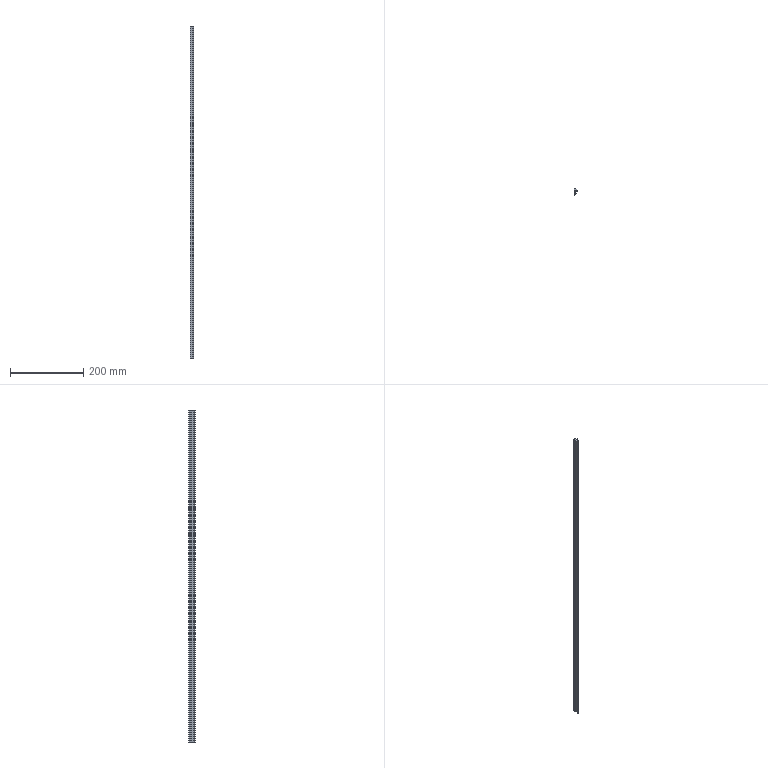Part | SolidWorks | features BaseBody 1, MoveFace 1 | 1 solid | 20 faces | box 10.8 x 17.5 x 907 mm | volume 71472 mm3 | cylinder 11 | plane 9 | commonest cylinder face diameters 1.6 x2 14 x2 0.4 x1 0.6 x1 0.8 x1 2.6 x1
STEP:
#1=CARTESIAN_POINT('',(-3.236,-11.055,807.));
#2=VERTEX_POINT('',#1);
#3=CARTESIAN_POINT('',(-4.3,-10.3,807.));
#4=VERTEX_POINT('',#3);
#5=CARTESIAN_POINT('',(-3.5,-10.3,807.));
#6=DIRECTION('',(0.,0.,-1.));
#7=DIRECTION('',(1.,0.,0.));
#8=AXIS2_PLACEMENT_3D('',#5,#6,#7);
#9=CIRCLE('',#8,0.8);
#10=EDGE_CURVE('',#2,#4,#9,.T.);
#11=ORIENTED_EDGE('',*,*,#10,.T.);
#12=CARTESIAN_POINT('',(-4.3,-10.3,-100.));
#13=VERTEX_POINT('',#12);
#14=CARTESIAN_POINT('',(-4.3,-10.3,-100.));
#15=DIRECTION('',(0.,0.,-1.));
#16=VECTOR('',#15,1000.);
#17=LINE('',#14,#16);
#18=EDGE_CURVE('',#4,#13,#17,.T.);
#19=ORIENTED_EDGE('',*,*,#18,.T.);
#20=CARTESIAN_POINT('',(-3.236,-11.055,-100.));
#21=VERTEX_POINT('',#20);
#22=CARTESIAN_POINT('',(-3.5,-10.3,-100.));
#23=DIRECTION('',(0.,0.,1.));
#24=DIRECTION('',(-1.,0.,0.));
#25=AXIS2_PLACEMENT_3D('',#22,#23,#24);
#26=CIRCLE('',#25,0.8);
#27=EDGE_CURVE('',#13,#21,#26,.T.);
#28=ORIENTED_EDGE('',*,*,#27,.T.);
#29=CARTESIAN_POINT('',(-3.236,-11.055,-100.));
#30=DIRECTION('',(0.,0.,-1.));
#31=VECTOR('',#30,1000.);
#32=LINE('',#29,#31);
#33=EDGE_CURVE('',#2,#21,#32,.T.);
#34=ORIENTED_EDGE('',*,*,#33,.F.);
#35=EDGE_LOOP('',(#11,#19,#28,#34));
#36=FACE_OUTER_BOUND('',#35,.T.);
#37=CARTESIAN_POINT('',(-3.5,-10.3,-100.));
#38=DIRECTION('',(0.,0.,-1.));
#39=DIRECTION('',(-1.,0.,0.));
#40=AXIS2_PLACEMENT_3D('',#37,#38,#39);
#41=CYLINDRICAL_SURFACE('',#40,0.8);
#42=ADVANCED_FACE('',(#36),#41,.T.);
#43=CARTESIAN_POINT('',(1.184,-6.397,-100.));
#44=VERTEX_POINT('',#43);
#45=CARTESIAN_POINT('',(-5.702,-4.29,-100.));
#46=DIRECTION('',(0.,0.,1.));
#47=DIRECTION('',(-1.,0.,0.));
#48=AXIS2_PLACEMENT_3D('',#45,#46,#47);
#49=CIRCLE('',#48,7.201);
#50=EDGE_CURVE('',#21,#44,#49,.T.);
#51=ORIENTED_EDGE('',*,*,#50,.T.);
#52=CARTESIAN_POINT('',(1.184,-6.397,807.));
#53=VERTEX_POINT('',#52);
#54=CARTESIAN_POINT('',(1.184,-6.397,-100.));
#55=DIRECTION('',(0.,0.,1.));
#56=VECTOR('',#55,1000.);
#57=LINE('',#54,#56);
#58=EDGE_CURVE('',#44,#53,#57,.T.);
#59=ORIENTED_EDGE('',*,*,#58,.T.);
#60=CARTESIAN_POINT('',(-5.702,-4.29,807.));
#61=DIRECTION('',(0.,0.,-1.));
#62=DIRECTION('',(1.,0.,0.));
#63=AXIS2_PLACEMENT_3D('',#60,#61,#62);
#64=CIRCLE('',#63,7.201);
#65=EDGE_CURVE('',#53,#2,#64,.T.);
#66=ORIENTED_EDGE('',*,*,#65,.T.);
#67=ORIENTED_EDGE('',*,*,#33,.T.);
#68=EDGE_LOOP('',(#51,#59,#66,#67));
#69=FACE_OUTER_BOUND('',#68,.T.);
#70=CARTESIAN_POINT('',(-5.702,-4.29,-100.));
#71=DIRECTION('',(0.,0.,-1.));
#72=DIRECTION('',(-1.,0.,0.));
#73=AXIS2_PLACEMENT_3D('',#70,#71,#72);
#74=CYLINDRICAL_SURFACE('',#73,7.201);
#75=ADVANCED_FACE('',(#69),#74,.T.);
#76=CARTESIAN_POINT('',(0.9,-6.,-100.));
#77=VERTEX_POINT('',#76);
#78=CARTESIAN_POINT('',(0.9,-6.3,-100.));
#79=DIRECTION('',(0.,0.,1.));
#80=DIRECTION('',(-1.,0.,0.));
#81=AXIS2_PLACEMENT_3D('',#78,#79,#80);
#82=CIRCLE('',#81,0.3);
#83=EDGE_CURVE('',#44,#77,#82,.T.);
#84=ORIENTED_EDGE('',*,*,#83,.T.);
#85=CARTESIAN_POINT('',(0.9,-6.,807.));
#86=VERTEX_POINT('',#85);
#87=CARTESIAN_POINT('',(0.9,-6.,-100.));
#88=DIRECTION('',(0.,0.,1.));
#89=VECTOR('',#88,1000.);
#90=LINE('',#87,#89);
#91=EDGE_CURVE('',#77,#86,#90,.T.);
#92=ORIENTED_EDGE('',*,*,#91,.T.);
#93=CARTESIAN_POINT('',(0.9,-6.3,807.));
#94=DIRECTION('',(0.,0.,-1.));
#95=DIRECTION('',(1.,0.,0.));
#96=AXIS2_PLACEMENT_3D('',#93,#94,#95);
#97=CIRCLE('',#96,0.3);
#98=EDGE_CURVE('',#86,#53,#97,.T.);
#99=ORIENTED_EDGE('',*,*,#98,.T.);
#100=ORIENTED_EDGE('',*,*,#58,.F.);
#101=EDGE_LOOP('',(#84,#92,#99,#100));
#102=FACE_OUTER_BOUND('',#101,.T.);
#103=CARTESIAN_POINT('',(0.9,-6.3,-100.));
#104=DIRECTION('',(0.,0.,-1.));
#105=DIRECTION('',(-1.,0.,0.));
#106=AXIS2_PLACEMENT_3D('',#103,#104,#105);
#107=CYLINDRICAL_SURFACE('',#106,0.3);
#108=ADVANCED_FACE('',(#102),#107,.T.);
#109=CARTESIAN_POINT('',(-2.5,-0.5,-100.));
#110=VERTEX_POINT('',#109);
#111=CARTESIAN_POINT('',(-2.5,-6.153,-100.));
#112=VERTEX_POINT('',#111);
#113=CARTESIAN_POINT('',(-2.5,-6.397,-100.));
#114=DIRECTION('',(0.,-1.,0.));
#115=VECTOR('',#114,1000.);
#116=LINE('',#113,#115);
#117=EDGE_CURVE('',#110,#112,#116,.T.);
#118=ORIENTED_EDGE('',*,*,#117,.F.);
#119=CARTESIAN_POINT('',(-4.2,1.695,-100.));
#120=VERTEX_POINT('',#119);
#121=CARTESIAN_POINT('',(-1.701,1.875,-100.));
#122=DIRECTION('',(0.,0.,1.));
#123=DIRECTION('',(-1.,0.,0.));
#124=AXIS2_PLACEMENT_3D('',#121,#122,#123);
#125=CIRCLE('',#124,2.506);
#126=EDGE_CURVE('',#120,#110,#125,.T.);
#127=ORIENTED_EDGE('',*,*,#126,.F.);
#128=CARTESIAN_POINT('',(-4.2,5.1,-100.));
#129=VERTEX_POINT('',#128);
#130=CARTESIAN_POINT('',(-4.2,-6.397,-100.));
#131=DIRECTION('',(0.,-1.,0.));
#132=VECTOR('',#131,1000.);
#133=LINE('',#130,#132);
#134=EDGE_CURVE('',#129,#120,#133,.T.);
#135=ORIENTED_EDGE('',*,*,#134,.F.);
#136=CARTESIAN_POINT('',(-2.892,6.4,-100.));
#137=VERTEX_POINT('',#136);
#138=CARTESIAN_POINT('',(-2.9,5.1,-100.));
#139=DIRECTION('',(0.,0.,1.));
#140=DIRECTION('',(-1.,0.,0.));
#141=AXIS2_PLACEMENT_3D('',#138,#139,#140);
#142=CIRCLE('',#141,1.3);
#143=EDGE_CURVE('',#137,#129,#142,.T.);
#144=ORIENTED_EDGE('',*,*,#143,.F.);
#145=CARTESIAN_POINT('',(0.5,5.5,-100.));
#146=VERTEX_POINT('',#145);
#147=CARTESIAN_POINT('',(-2.934,-0.5999,-100.));
#148=DIRECTION('',(0.,0.,1.));
#149=DIRECTION('',(-1.,0.,0.));
#150=AXIS2_PLACEMENT_3D('',#147,#148,#149);
#151=CIRCLE('',#150,7.);
#152=EDGE_CURVE('',#146,#137,#151,.T.);
#153=ORIENTED_EDGE('',*,*,#152,.F.);
#154=CARTESIAN_POINT('',(5.5,1.7,-100.));
#155=VERTEX_POINT('',#154);
#156=CARTESIAN_POINT('',(5.5,1.7,-100.));
#157=DIRECTION('',(-0.7962,0.6051,0.));
#158=VECTOR('',#157,1000.);
#159=LINE('',#156,#158);
#160=EDGE_CURVE('',#155,#146,#159,.T.);
#161=ORIENTED_EDGE('',*,*,#160,.F.);
#162=CARTESIAN_POINT('',(6.458,-0.2215,-100.));
#163=VERTEX_POINT('',#162);
#164=CARTESIAN_POINT('',(6.458,-0.2215,-100.));
#165=DIRECTION('',(-0.4462,0.8949,0.));
#166=VECTOR('',#165,1000.);
#167=LINE('',#164,#166);
#168=EDGE_CURVE('',#163,#155,#167,.T.);
#169=ORIENTED_EDGE('',*,*,#168,.F.);
#170=CARTESIAN_POINT('',(5.895,-0.7433,-100.));
#171=VERTEX_POINT('',#170);
#172=CARTESIAN_POINT('',(6.1,-0.4,-100.));
#173=DIRECTION('',(0.,0.,1.));
#174=DIRECTION('',(-1.,0.,0.));
#175=AXIS2_PLACEMENT_3D('',#172,#173,#174);
#176=CIRCLE('',#175,0.4);
#177=EDGE_CURVE('',#171,#163,#176,.T.);
#178=ORIENTED_EDGE('',*,*,#177,.F.);
#179=CARTESIAN_POINT('',(3.,0.,-100.));
#180=VERTEX_POINT('',#179);
#181=CARTESIAN_POINT('',(2.746,-6.995,-100.));
#182=DIRECTION('',(0.,0.,-1.));
#183=DIRECTION('',(-1.,0.,0.));
#184=AXIS2_PLACEMENT_3D('',#181,#182,#183);
#185=CIRCLE('',#184,7.);
#186=EDGE_CURVE('',#180,#171,#185,.T.);
#187=ORIENTED_EDGE('',*,*,#186,.F.);
#188=CARTESIAN_POINT('',(0.,0.,-100.));
#189=VERTEX_POINT('',#188);
#190=CARTESIAN_POINT('',(-6.814,0.,-100.));
#191=DIRECTION('',(1.,0.,0.));
#192=VECTOR('',#191,1000.);
#193=LINE('',#190,#192);
#194=EDGE_CURVE('',#189,#180,#193,.T.);
#195=ORIENTED_EDGE('',*,*,#194,.F.);
#196=CARTESIAN_POINT('',(0.,-5.8,-100.));
#197=VERTEX_POINT('',#196);
#198=CARTESIAN_POINT('',(0.,-6.397,-100.));
#199=DIRECTION('',(0.,1.,0.));
#200=VECTOR('',#199,1000.);
#201=LINE('',#198,#200);
#202=EDGE_CURVE('',#197,#189,#201,.T.);
#203=ORIENTED_EDGE('',*,*,#202,.F.);
#204=CARTESIAN_POINT('',(0.2,-6.,-100.));
#205=VERTEX_POINT('',#204);
#206=CARTESIAN_POINT('',(0.2,-5.8,-100.));
#207=DIRECTION('',(0.,0.,1.));
#208=DIRECTION('',(-1.,0.,0.));
#209=AXIS2_PLACEMENT_3D('',#206,#207,#208);
#210=CIRCLE('',#209,0.2);
#211=EDGE_CURVE('',#197,#205,#210,.T.);
#212=ORIENTED_EDGE('',*,*,#211,.T.);
#213=CARTESIAN_POINT('',(-6.814,-6.,-100.));
#214=DIRECTION('',(-1.,0.,0.));
#215=VECTOR('',#214,1000.);
#216=LINE('',#213,#215);
#217=EDGE_CURVE('',#77,#205,#216,.T.);
#218=ORIENTED_EDGE('',*,*,#217,.F.);
#219=ORIENTED_EDGE('',*,*,#83,.F.);
#220=ORIENTED_EDGE('',*,*,#50,.F.);
#221=ORIENTED_EDGE('',*,*,#27,.F.);
#222=CARTESIAN_POINT('',(-3.998,-9.674,-100.));
#223=VERTEX_POINT('',#222);
#224=CARTESIAN_POINT('',(-3.5,-10.3,-100.));
#225=DIRECTION('',(0.,0.,1.));
#226=DIRECTION('',(-1.,0.,0.));
#227=AXIS2_PLACEMENT_3D('',#224,#225,#226);
#228=CIRCLE('',#227,0.8);
#229=EDGE_CURVE('',#223,#13,#228,.T.);
#230=ORIENTED_EDGE('',*,*,#229,.F.);
#231=CARTESIAN_POINT('',(-6.814,-6.397,-100.));
#232=DIRECTION('',(0.,0.,-1.));
#233=DIRECTION('',(-1.,0.,0.));
#234=AXIS2_PLACEMENT_3D('',#231,#232,#233);
#235=CIRCLE('',#234,4.321);
#236=EDGE_CURVE('',#112,#223,#235,.T.);
#237=ORIENTED_EDGE('',*,*,#236,.F.);
#238=EDGE_LOOP('',(#118,#127,#135,#144,#153,#161,#169,#178,#187,#195,#203,#212,#218,#219,#220,#221,#230,#237));
#239=FACE_OUTER_BOUND('',#238,.T.);
#240=CARTESIAN_POINT('',(-6.814,-6.397,-100.));
#241=DIRECTION('',(0.,0.,1.));
#242=DIRECTION('',(1.,0.,0.));
#243=AXIS2_PLACEMENT_3D('',#240,#241,#242);
#244=PLANE('',#243);
#245=ADVANCED_FACE('',(#239),#244,.F.);
#246=ORIENTED_EDGE('',*,*,#18,.F.);
#247=CARTESIAN_POINT('',(-3.998,-9.674,807.));
#248=VERTEX_POINT('',#247);
#249=CARTESIAN_POINT('',(-3.5,-10.3,807.));
#250=DIRECTION('',(0.,0.,-1.));
#251=DIRECTION('',(1.,0.,0.));
#252=AXIS2_PLACEMENT_3D('',#249,#250,#251);
#253=CIRCLE('',#252,0.8);
#254=EDGE_CURVE('',#4,#248,#253,.T.);
#255=ORIENTED_EDGE('',*,*,#254,.T.);
#256=CARTESIAN_POINT('',(-3.998,-9.674,-100.));
#257=DIRECTION('',(0.,0.,-1.));
#258=VECTOR('',#257,1000.);
#259=LINE('',#256,#258);
#260=EDGE_CURVE('',#248,#223,#259,.T.);
#261=ORIENTED_EDGE('',*,*,#260,.T.);
#262=ORIENTED_EDGE('',*,*,#229,.T.);
#263=EDGE_LOOP('',(#246,#255,#261,#262));
#264=FACE_OUTER_BOUND('',#263,.T.);
#265=CARTESIAN_POINT('',(-3.5,-10.3,-100.));
#266=DIRECTION('',(0.,0.,-1.));
#267=DIRECTION('',(-1.,0.,0.));
#268=AXIS2_PLACEMENT_3D('',#265,#266,#267);
#269=CYLINDRICAL_SURFACE('',#268,0.8);
#270=ADVANCED_FACE('',(#264),#269,.T.);
#271=CARTESIAN_POINT('',(-4.2,1.695,807.));
#272=VERTEX_POINT('',#271);
#273=CARTESIAN_POINT('',(-2.5,-0.5,807.));
#274=VERTEX_POINT('',#273);
#275=CARTESIAN_POINT('',(-1.701,1.875,807.));
#276=DIRECTION('',(0.,0.,1.));
#277=DIRECTION('',(1.,0.,0.));
#278=AXIS2_PLACEMENT_3D('',#275,#276,#277);
#279=CIRCLE('',#278,2.506);
#280=EDGE_CURVE('',#272,#274,#279,.T.);
#281=ORIENTED_EDGE('',*,*,#280,.T.);
#282=CARTESIAN_POINT('',(-2.5,-6.153,807.));
#283=VERTEX_POINT('',#282);
#284=CARTESIAN_POINT('',(-2.5,-6.397,807.));
#285=DIRECTION('',(0.,-1.,0.));
#286=VECTOR('',#285,1000.);
#287=LINE('',#284,#286);
#288=EDGE_CURVE('',#274,#283,#287,.T.);
#289=ORIENTED_EDGE('',*,*,#288,.T.);
#290=CARTESIAN_POINT('',(-6.814,-6.397,807.));
#291=DIRECTION('',(0.,0.,-1.));
#292=DIRECTION('',(1.,0.,0.));
#293=AXIS2_PLACEMENT_3D('',#290,#291,#292);
#294=CIRCLE('',#293,4.321);
#295=EDGE_CURVE('',#283,#248,#294,.T.);
#296=ORIENTED_EDGE('',*,*,#295,.T.);
#297=ORIENTED_EDGE('',*,*,#254,.F.);
#298=ORIENTED_EDGE('',*,*,#10,.F.);
#299=ORIENTED_EDGE('',*,*,#65,.F.);
#300=ORIENTED_EDGE('',*,*,#98,.F.);
#301=CARTESIAN_POINT('',(0.2,-6.,807.));
#302=VERTEX_POINT('',#301);
#303=CARTESIAN_POINT('',(-6.814,-6.,807.));
#304=DIRECTION('',(-1.,0.,0.));
#305=VECTOR('',#304,1000.);
#306=LINE('',#303,#305);
#307=EDGE_CURVE('',#86,#302,#306,.T.);
#308=ORIENTED_EDGE('',*,*,#307,.T.);
#309=CARTESIAN_POINT('',(0.,-5.8,807.));
#310=VERTEX_POINT('',#309);
#311=CARTESIAN_POINT('',(0.2,-5.8,807.));
#312=DIRECTION('',(0.,0.,-1.));
#313=DIRECTION('',(1.,0.,0.));
#314=AXIS2_PLACEMENT_3D('',#311,#312,#313);
#315=CIRCLE('',#314,0.2);
#316=EDGE_CURVE('',#302,#310,#315,.T.);
#317=ORIENTED_EDGE('',*,*,#316,.T.);
#318=CARTESIAN_POINT('',(0.,0.,807.));
#319=VERTEX_POINT('',#318);
#320=CARTESIAN_POINT('',(0.,-6.397,807.));
#321=DIRECTION('',(0.,1.,0.));
#322=VECTOR('',#321,1000.);
#323=LINE('',#320,#322);
#324=EDGE_CURVE('',#310,#319,#323,.T.);
#325=ORIENTED_EDGE('',*,*,#324,.T.);
#326=CARTESIAN_POINT('',(3.,0.,807.));
#327=VERTEX_POINT('',#326);
#328=CARTESIAN_POINT('',(-6.814,0.,807.));
#329=DIRECTION('',(1.,0.,0.));
#330=VECTOR('',#329,1000.);
#331=LINE('',#328,#330);
#332=EDGE_CURVE('',#319,#327,#331,.T.);
#333=ORIENTED_EDGE('',*,*,#332,.T.);
#334=CARTESIAN_POINT('',(5.895,-0.7433,807.));
#335=VERTEX_POINT('',#334);
#336=CARTESIAN_POINT('',(2.746,-6.995,807.));
#337=DIRECTION('',(0.,0.,-1.));
#338=DIRECTION('',(1.,0.,0.));
#339=AXIS2_PLACEMENT_3D('',#336,#337,#338);
#340=CIRCLE('',#339,7.);
#341=EDGE_CURVE('',#327,#335,#340,.T.);
#342=ORIENTED_EDGE('',*,*,#341,.T.);
#343=CARTESIAN_POINT('',(6.458,-0.2215,807.));
#344=VERTEX_POINT('',#343);
#345=CARTESIAN_POINT('',(6.1,-0.4,807.));
#346=DIRECTION('',(0.,0.,-1.));
#347=DIRECTION('',(1.,0.,0.));
#348=AXIS2_PLACEMENT_3D('',#345,#346,#347);
#349=CIRCLE('',#348,0.4);
#350=EDGE_CURVE('',#344,#335,#349,.T.);
#351=ORIENTED_EDGE('',*,*,#350,.F.);
#352=CARTESIAN_POINT('',(5.5,1.7,807.));
#353=VERTEX_POINT('',#352);
#354=CARTESIAN_POINT('',(6.282,0.1323,807.));
#355=DIRECTION('',(-0.4462,0.8949,0.));
#356=VECTOR('',#355,1000.);
#357=LINE('',#354,#356);
#358=EDGE_CURVE('',#344,#353,#357,.T.);
#359=ORIENTED_EDGE('',*,*,#358,.T.);
#360=CARTESIAN_POINT('',(0.5,5.5,807.));
#361=VERTEX_POINT('',#360);
#362=CARTESIAN_POINT('',(1.595,4.668,807.));
#363=DIRECTION('',(-0.7962,0.6051,0.));
#364=VECTOR('',#363,1000.);
#365=LINE('',#362,#364);
#366=EDGE_CURVE('',#353,#361,#365,.T.);
#367=ORIENTED_EDGE('',*,*,#366,.T.);
#368=CARTESIAN_POINT('',(-2.892,6.4,807.));
#369=VERTEX_POINT('',#368);
#370=CARTESIAN_POINT('',(-2.934,-0.5999,807.));
#371=DIRECTION('',(0.,0.,1.));
#372=DIRECTION('',(1.,0.,0.));
#373=AXIS2_PLACEMENT_3D('',#370,#371,#372);
#374=CIRCLE('',#373,7.);
#375=EDGE_CURVE('',#361,#369,#374,.T.);
#376=ORIENTED_EDGE('',*,*,#375,.T.);
#377=CARTESIAN_POINT('',(-4.2,5.1,807.));
#378=VERTEX_POINT('',#377);
#379=CARTESIAN_POINT('',(-2.9,5.1,807.));
#380=DIRECTION('',(0.,0.,1.));
#381=DIRECTION('',(1.,0.,0.));
#382=AXIS2_PLACEMENT_3D('',#379,#380,#381);
#383=CIRCLE('',#382,1.3);
#384=EDGE_CURVE('',#369,#378,#383,.T.);
#385=ORIENTED_EDGE('',*,*,#384,.T.);
#386=CARTESIAN_POINT('',(-4.2,-6.397,807.));
#387=DIRECTION('',(0.,-1.,0.));
#388=VECTOR('',#387,1000.);
#389=LINE('',#386,#388);
#390=EDGE_CURVE('',#378,#272,#389,.T.);
#391=ORIENTED_EDGE('',*,*,#390,.T.);
#392=EDGE_LOOP('',(#281,#289,#296,#297,#298,#299,#300,#308,#317,#325,#333,#342,#351,#359,#367,#376,#385,#391));
#393=FACE_OUTER_BOUND('',#392,.T.);
#394=CARTESIAN_POINT('',(-6.814,-6.397,807.));
#395=DIRECTION('',(0.,0.,1.));
#396=DIRECTION('',(1.,0.,0.));
#397=AXIS2_PLACEMENT_3D('',#394,#395,#396);
#398=PLANE('',#397);
#399=ADVANCED_FACE('',(#393),#398,.T.);
#400=ORIENTED_EDGE('',*,*,#217,.T.);
#401=CARTESIAN_POINT('',(0.2,-6.,-100.));
#402=DIRECTION('',(0.,0.,1.));
#403=VECTOR('',#402,1000.);
#404=LINE('',#401,#403);
#405=EDGE_CURVE('',#205,#302,#404,.T.);
#406=ORIENTED_EDGE('',*,*,#405,.T.);
#407=ORIENTED_EDGE('',*,*,#307,.F.);
#408=ORIENTED_EDGE('',*,*,#91,.F.);
#409=EDGE_LOOP('',(#400,#406,#407,#408));
#410=FACE_OUTER_BOUND('',#409,.T.);
#411=CARTESIAN_POINT('',(0.9,-6.,-100.));
#412=DIRECTION('',(0.,1.,0.));
#413=DIRECTION('',(0.,0.,1.));
#414=AXIS2_PLACEMENT_3D('',#411,#412,#413);
#415=PLANE('',#414);
#416=ADVANCED_FACE('',(#410),#415,.T.);
#417=CARTESIAN_POINT('',(-2.5,-6.153,-100.));
#418=DIRECTION('',(0.,0.,1.));
#419=VECTOR('',#418,1000.);
#420=LINE('',#417,#419);
#421=EDGE_CURVE('',#112,#283,#420,.T.);
#422=ORIENTED_EDGE('',*,*,#421,.F.);
#423=ORIENTED_EDGE('',*,*,#236,.T.);
#424=ORIENTED_EDGE('',*,*,#260,.F.);
#425=ORIENTED_EDGE('',*,*,#295,.F.);
#426=EDGE_LOOP('',(#422,#423,#424,#425));
#427=FACE_OUTER_BOUND('',#426,.T.);
#428=CARTESIAN_POINT('',(-6.814,-6.397,-100.));
#429=DIRECTION('',(0.,0.,-1.));
#430=DIRECTION('',(-1.,0.,0.));
#431=AXIS2_PLACEMENT_3D('',#428,#429,#430);
#432=CYLINDRICAL_SURFACE('',#431,4.321);
#433=ADVANCED_FACE('',(#427),#432,.F.);
#434=ORIENTED_EDGE('',*,*,#117,.T.);
#435=ORIENTED_EDGE('',*,*,#421,.T.);
#436=ORIENTED_EDGE('',*,*,#288,.F.);
#437=CARTESIAN_POINT('',(-2.5,-0.5,-100.));
#438=DIRECTION('',(0.,0.,-1.));
#439=VECTOR('',#438,1000.);
#440=LINE('',#437,#439);
#441=EDGE_CURVE('',#274,#110,#440,.T.);
#442=ORIENTED_EDGE('',*,*,#441,.T.);
#443=EDGE_LOOP('',(#434,#435,#436,#442));
#444=FACE_OUTER_BOUND('',#443,.T.);
#445=CARTESIAN_POINT('',(-2.5,-0.5,-100.));
#446=DIRECTION('',(-1.,0.,0.));
#447=DIRECTION('',(0.,0.,1.));
#448=AXIS2_PLACEMENT_3D('',#445,#446,#447);
#449=PLANE('',#448);
#450=ADVANCED_FACE('',(#444),#449,.T.);
#451=ORIENTED_EDGE('',*,*,#126,.T.);
#452=ORIENTED_EDGE('',*,*,#441,.F.);
#453=ORIENTED_EDGE('',*,*,#280,.F.);
#454=CARTESIAN_POINT('',(-4.2,1.695,-100.));
#455=DIRECTION('',(0.,0.,-1.));
#456=VECTOR('',#455,1000.);
#457=LINE('',#454,#456);
#458=EDGE_CURVE('',#272,#120,#457,.T.);
#459=ORIENTED_EDGE('',*,*,#458,.T.);
#460=EDGE_LOOP('',(#451,#452,#453,#459));
#461=FACE_OUTER_BOUND('',#460,.T.);
#462=CARTESIAN_POINT('',(-1.701,1.875,-100.));
#463=DIRECTION('',(0.,0.,-1.));
#464=DIRECTION('',(-1.,0.,0.));
#465=AXIS2_PLACEMENT_3D('',#462,#463,#464);
#466=CYLINDRICAL_SURFACE('',#465,2.506);
#467=ADVANCED_FACE('',(#461),#466,.T.);
#468=ORIENTED_EDGE('',*,*,#134,.T.);
#469=ORIENTED_EDGE('',*,*,#458,.F.);
#470=ORIENTED_EDGE('',*,*,#390,.F.);
#471=CARTESIAN_POINT('',(-4.2,5.1,-100.));
#472=DIRECTION('',(0.,0.,-1.));
#473=VECTOR('',#472,1000.);
#474=LINE('',#471,#473);
#475=EDGE_CURVE('',#378,#129,#474,.T.);
#476=ORIENTED_EDGE('',*,*,#475,.T.);
#477=EDGE_LOOP('',(#468,#469,#470,#476));
#478=FACE_OUTER_BOUND('',#477,.T.);
#479=CARTESIAN_POINT('',(-4.2,5.1,-100.));
#480=DIRECTION('',(-1.,0.,0.));
#481=DIRECTION('',(0.,0.,1.));
#482=AXIS2_PLACEMENT_3D('',#479,#480,#481);
#483=PLANE('',#482);
#484=ADVANCED_FACE('',(#478),#483,.T.);
#485=ORIENTED_EDGE('',*,*,#143,.T.);
#486=ORIENTED_EDGE('',*,*,#475,.F.);
#487=ORIENTED_EDGE('',*,*,#384,.F.);
#488=CARTESIAN_POINT('',(-2.892,6.4,-100.));
#489=DIRECTION('',(0.,0.,-1.));
#490=VECTOR('',#489,1000.);
#491=LINE('',#488,#490);
#492=EDGE_CURVE('',#369,#137,#491,.T.);
#493=ORIENTED_EDGE('',*,*,#492,.T.);
#494=EDGE_LOOP('',(#485,#486,#487,#493));
#495=FACE_OUTER_BOUND('',#494,.T.);
#496=CARTESIAN_POINT('',(-2.9,5.1,-100.));
#497=DIRECTION('',(0.,0.,-1.));
#498=DIRECTION('',(-1.,0.,0.));
#499=AXIS2_PLACEMENT_3D('',#496,#497,#498);
#500=CYLINDRICAL_SURFACE('',#499,1.3);
#501=ADVANCED_FACE('',(#495),#500,.T.);
#502=ORIENTED_EDGE('',*,*,#152,.T.);
#503=ORIENTED_EDGE('',*,*,#492,.F.);
#504=ORIENTED_EDGE('',*,*,#375,.F.);
#505=CARTESIAN_POINT('',(0.5,5.5,-100.));
#506=DIRECTION('',(0.,0.,-1.));
#507=VECTOR('',#506,1000.);
#508=LINE('',#505,#507);
#509=EDGE_CURVE('',#361,#146,#508,.T.);
#510=ORIENTED_EDGE('',*,*,#509,.T.);
#511=EDGE_LOOP('',(#502,#503,#504,#510));
#512=FACE_OUTER_BOUND('',#511,.T.);
#513=CARTESIAN_POINT('',(-2.934,-0.5999,-100.));
#514=DIRECTION('',(0.,0.,-1.));
#515=DIRECTION('',(-1.,0.,0.));
#516=AXIS2_PLACEMENT_3D('',#513,#514,#515);
#517=CYLINDRICAL_SURFACE('',#516,7.);
#518=ADVANCED_FACE('',(#512),#517,.T.);
#519=ORIENTED_EDGE('',*,*,#160,.T.);
#520=ORIENTED_EDGE('',*,*,#509,.F.);
#521=ORIENTED_EDGE('',*,*,#366,.F.);
#522=CARTESIAN_POINT('',(5.5,1.7,-100.));
#523=DIRECTION('',(0.,0.,-1.));
#524=VECTOR('',#523,1000.);
#525=LINE('',#522,#524);
#526=EDGE_CURVE('',#353,#155,#525,.T.);
#527=ORIENTED_EDGE('',*,*,#526,.T.);
#528=EDGE_LOOP('',(#519,#520,#521,#527));
#529=FACE_OUTER_BOUND('',#528,.T.);
#530=CARTESIAN_POINT('',(5.5,1.7,-100.));
#531=DIRECTION('',(0.6051,0.7962,0.));
#532=DIRECTION('',(-0.7962,0.6051,0.));
#533=AXIS2_PLACEMENT_3D('',#530,#531,#532);
#534=PLANE('',#533);
#535=ADVANCED_FACE('',(#529),#534,.T.);
#536=ORIENTED_EDGE('',*,*,#168,.T.);
#537=ORIENTED_EDGE('',*,*,#526,.F.);
#538=ORIENTED_EDGE('',*,*,#358,.F.);
#539=CARTESIAN_POINT('',(6.458,-0.2215,-100.));
#540=DIRECTION('',(0.,0.,-1.));
#541=VECTOR('',#540,1000.);
#542=LINE('',#539,#541);
#543=EDGE_CURVE('',#344,#163,#542,.T.);
#544=ORIENTED_EDGE('',*,*,#543,.T.);
#545=EDGE_LOOP('',(#536,#537,#538,#544));
#546=FACE_OUTER_BOUND('',#545,.T.);
#547=CARTESIAN_POINT('',(6.458,-0.2215,-100.));
#548=DIRECTION('',(0.8949,0.4462,0.));
#549=DIRECTION('',(-0.4462,0.8949,0.));
#550=AXIS2_PLACEMENT_3D('',#547,#548,#549);
#551=PLANE('',#550);
#552=ADVANCED_FACE('',(#546),#551,.T.);
#553=CARTESIAN_POINT('',(3.,0.,-100.));
#554=DIRECTION('',(0.,0.,1.));
#555=VECTOR('',#554,1000.);
#556=LINE('',#553,#555);
#557=EDGE_CURVE('',#180,#327,#556,.T.);
#558=ORIENTED_EDGE('',*,*,#557,.F.);
#559=ORIENTED_EDGE('',*,*,#186,.T.);
#560=CARTESIAN_POINT('',(5.895,-0.7433,-100.));
#561=DIRECTION('',(0.,0.,-1.));
#562=VECTOR('',#561,1000.);
#563=LINE('',#560,#562);
#564=EDGE_CURVE('',#335,#171,#563,.T.);
#565=ORIENTED_EDGE('',*,*,#564,.F.);
#566=ORIENTED_EDGE('',*,*,#341,.F.);
#567=EDGE_LOOP('',(#558,#559,#565,#566));
#568=FACE_OUTER_BOUND('',#567,.T.);
#569=CARTESIAN_POINT('',(2.746,-6.995,-100.));
#570=DIRECTION('',(0.,0.,-1.));
#571=DIRECTION('',(-1.,0.,0.));
#572=AXIS2_PLACEMENT_3D('',#569,#570,#571);
#573=CYLINDRICAL_SURFACE('',#572,7.);
#574=ADVANCED_FACE('',(#568),#573,.F.);
#575=ORIENTED_EDGE('',*,*,#194,.T.);
#576=ORIENTED_EDGE('',*,*,#557,.T.);
#577=ORIENTED_EDGE('',*,*,#332,.F.);
#578=CARTESIAN_POINT('',(0.,0.,-100.));
#579=DIRECTION('',(0.,0.,-1.));
#580=VECTOR('',#579,1000.);
#581=LINE('',#578,#580);
#582=EDGE_CURVE('',#319,#189,#581,.T.);
#583=ORIENTED_EDGE('',*,*,#582,.T.);
#584=EDGE_LOOP('',(#575,#576,#577,#583));
#585=FACE_OUTER_BOUND('',#584,.T.);
#586=CARTESIAN_POINT('',(0.,0.,-100.));
#587=DIRECTION('',(0.,-1.,0.));
#588=DIRECTION('',(0.,0.,-1.));
#589=AXIS2_PLACEMENT_3D('',#586,#587,#588);
#590=PLANE('',#589);
#591=ADVANCED_FACE('',(#585),#590,.T.);
#592=ORIENTED_EDGE('',*,*,#202,.T.);
#593=ORIENTED_EDGE('',*,*,#582,.F.);
#594=ORIENTED_EDGE('',*,*,#324,.F.);
#595=CARTESIAN_POINT('',(0.,-5.8,-100.));
#596=DIRECTION('',(0.,0.,-1.));
#597=VECTOR('',#596,1000.);
#598=LINE('',#595,#597);
#599=EDGE_CURVE('',#310,#197,#598,.T.);
#600=ORIENTED_EDGE('',*,*,#599,.T.);
#601=EDGE_LOOP('',(#592,#593,#594,#600));
#602=FACE_OUTER_BOUND('',#601,.T.);
#603=CARTESIAN_POINT('',(0.,-5.8,-100.));
#604=DIRECTION('',(1.,0.,0.));
#605=DIRECTION('',(0.,0.,-1.));
#606=AXIS2_PLACEMENT_3D('',#603,#604,#605);
#607=PLANE('',#606);
#608=ADVANCED_FACE('',(#602),#607,.T.);
#609=ORIENTED_EDGE('',*,*,#405,.F.);
#610=ORIENTED_EDGE('',*,*,#211,.F.);
#611=ORIENTED_EDGE('',*,*,#599,.F.);
#612=ORIENTED_EDGE('',*,*,#316,.F.);
#613=EDGE_LOOP('',(#609,#610,#611,#612));
#614=FACE_OUTER_BOUND('',#613,.T.);
#615=CARTESIAN_POINT('',(0.2,-5.8,-100.));
#616=DIRECTION('',(0.,0.,-1.));
#617=DIRECTION('',(-1.,0.,0.));
#618=AXIS2_PLACEMENT_3D('',#615,#616,#617);
#619=CYLINDRICAL_SURFACE('',#618,0.2);
#620=ADVANCED_FACE('',(#614),#619,.F.);
#621=ORIENTED_EDGE('',*,*,#177,.T.);
#622=ORIENTED_EDGE('',*,*,#543,.F.);
#623=ORIENTED_EDGE('',*,*,#350,.T.);
#624=ORIENTED_EDGE('',*,*,#564,.T.);
#625=EDGE_LOOP('',(#621,#622,#623,#624));
#626=FACE_OUTER_BOUND('',#625,.T.);
#627=CARTESIAN_POINT('',(6.1,-0.4,-100.));
#628=DIRECTION('',(0.,0.,-1.));
#629=DIRECTION('',(-1.,0.,0.));
#630=AXIS2_PLACEMENT_3D('',#627,#628,#629);
#631=CYLINDRICAL_SURFACE('',#630,0.4);
#632=ADVANCED_FACE('',(#626),#631,.T.);
#633=CLOSED_SHELL('',(#42,#75,#108,#245,#270,#399,#416,#433,#450,#467,#484,#501,#518,#535,#552,#574,#591,#608,#620,#632));
#634=MANIFOLD_SOLID_BREP('',#633);
#635=CARTESIAN_POINT('',(0.,0.,0.));
#636=DIRECTION('',(0.,0.,1.));
#637=DIRECTION('',(1.,0.,0.));
#638=AXIS2_PLACEMENT_3D('',#635,#636,#637);
#639=(LENGTH_UNIT()NAMED_UNIT(*)SI_UNIT(.MILLI.,.METRE.));
#640=UNCERTAINTY_MEASURE_WITH_UNIT(LENGTH_MEASURE(0.00001),#639,'','');
#641=(NAMED_UNIT(*)PLANE_ANGLE_UNIT()SI_UNIT($,.RADIAN.));
#642=(NAMED_UNIT(*)SI_UNIT($,.STERADIAN.)SOLID_ANGLE_UNIT());
#643=(GEOMETRIC_REPRESENTATION_CONTEXT(3)GLOBAL_UNCERTAINTY_ASSIGNED_CONTEXT((#640))GLOBAL_UNIT_ASSIGNED_CONTEXT((#639,#641,#642))REPRESENTATION_CONTEXT('',''));
#644=ADVANCED_BREP_SHAPE_REPRESENTATION('',(#634,#638),#643);